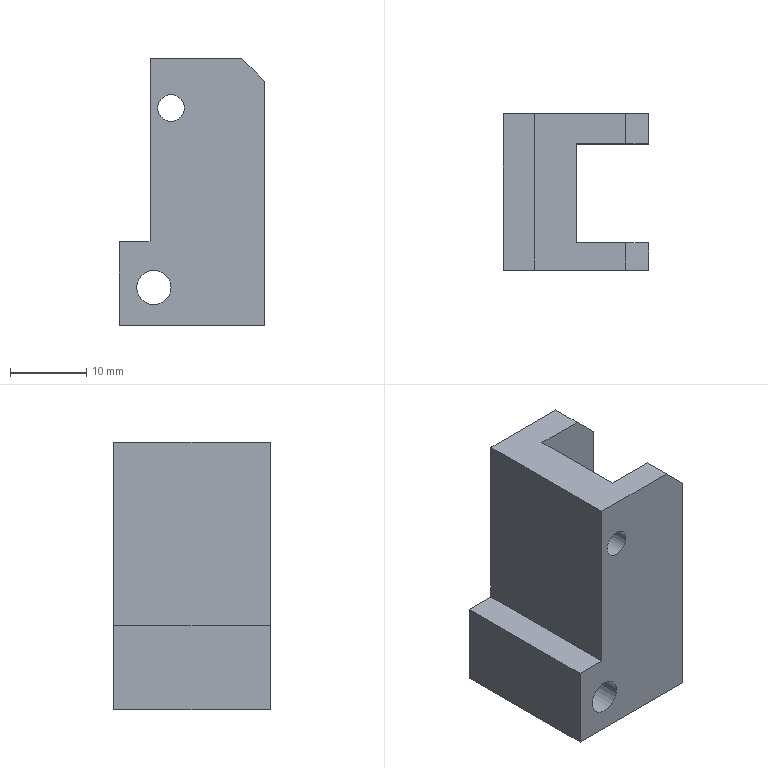Part | NX | 1 solid | 18 faces | box 19 x 20.5 x 35 mm | volume 6785 mm3 | plane 14 | cylinder 4 | commonest cylinder face diameters 3.5 x2 4.5 x2
STEP:
#1=CARTESIAN_POINT('',(9.5,16.55,0.));
#2=VERTEX_POINT('',#1);
#3=CARTESIAN_POINT('',(19.,16.55,0.));
#4=VERTEX_POINT('',#3);
#5=CARTESIAN_POINT('',(9.5,16.55,0.));
#6=DIRECTION('',(1.,0.,0.));
#7=VECTOR('',#6,1000.);
#8=LINE('',#5,#7);
#9=EDGE_CURVE('',#2,#4,#8,.T.);
#10=ORIENTED_EDGE('',*,*,#9,.F.);
#11=CARTESIAN_POINT('',(9.5,3.55,0.));
#12=VERTEX_POINT('',#11);
#13=CARTESIAN_POINT('',(9.5,3.55,0.));
#14=DIRECTION('',(0.,1.,0.));
#15=VECTOR('',#14,1000.);
#16=LINE('',#13,#15);
#17=EDGE_CURVE('',#12,#2,#16,.T.);
#18=ORIENTED_EDGE('',*,*,#17,.F.);
#19=CARTESIAN_POINT('',(19.,3.55,0.));
#20=VERTEX_POINT('',#19);
#21=CARTESIAN_POINT('',(9.5,3.55,0.));
#22=DIRECTION('',(1.,0.,0.));
#23=VECTOR('',#22,1000.);
#24=LINE('',#21,#23);
#25=EDGE_CURVE('',#12,#20,#24,.T.);
#26=ORIENTED_EDGE('',*,*,#25,.T.);
#27=CARTESIAN_POINT('',(19.,0.,0.));
#28=VERTEX_POINT('',#27);
#29=CARTESIAN_POINT('',(19.,3.55,0.));
#30=DIRECTION('',(0.,-1.,0.));
#31=VECTOR('',#30,1000.);
#32=LINE('',#29,#31);
#33=EDGE_CURVE('',#20,#28,#32,.T.);
#34=ORIENTED_EDGE('',*,*,#33,.T.);
#35=CARTESIAN_POINT('',(0.,0.,0.));
#36=VERTEX_POINT('',#35);
#37=CARTESIAN_POINT('',(19.,0.,0.));
#38=DIRECTION('',(-1.,0.,0.));
#39=VECTOR('',#38,1000.);
#40=LINE('',#37,#39);
#41=EDGE_CURVE('',#28,#36,#40,.T.);
#42=ORIENTED_EDGE('',*,*,#41,.T.);
#43=CARTESIAN_POINT('',(0.,20.5,0.));
#44=VERTEX_POINT('',#43);
#45=CARTESIAN_POINT('',(0.,0.,0.));
#46=DIRECTION('',(0.,1.,0.));
#47=VECTOR('',#46,1000.);
#48=LINE('',#45,#47);
#49=EDGE_CURVE('',#36,#44,#48,.T.);
#50=ORIENTED_EDGE('',*,*,#49,.T.);
#51=CARTESIAN_POINT('',(19.,20.5,0.));
#52=VERTEX_POINT('',#51);
#53=CARTESIAN_POINT('',(0.,20.5,0.));
#54=DIRECTION('',(1.,0.,0.));
#55=VECTOR('',#54,1000.);
#56=LINE('',#53,#55);
#57=EDGE_CURVE('',#44,#52,#56,.T.);
#58=ORIENTED_EDGE('',*,*,#57,.T.);
#59=CARTESIAN_POINT('',(19.,20.5,0.));
#60=DIRECTION('',(0.,-1.,0.));
#61=VECTOR('',#60,1000.);
#62=LINE('',#59,#61);
#63=EDGE_CURVE('',#52,#4,#62,.T.);
#64=ORIENTED_EDGE('',*,*,#63,.T.);
#65=EDGE_LOOP('',(#10,#18,#26,#34,#42,#50,#58,#64));
#66=FACE_BOUND('',#65,.T.);
#67=CARTESIAN_POINT('',(0.,0.,0.));
#68=DIRECTION('',(0.,0.,1.));
#69=DIRECTION('',(1.,0.,0.));
#70=AXIS2_PLACEMENT_3D('',#67,#68,#69);
#71=PLANE('',#70);
#72=ADVANCED_FACE('',(#66),#71,.F.);
#73=ORIENTED_EDGE('',*,*,#9,.T.);
#74=CARTESIAN_POINT('',(19.,16.55,32.));
#75=VERTEX_POINT('',#74);
#76=CARTESIAN_POINT('',(19.,16.55,32.));
#77=DIRECTION('',(0.,0.,-1.));
#78=VECTOR('',#77,1000.);
#79=LINE('',#76,#78);
#80=EDGE_CURVE('',#75,#4,#79,.T.);
#81=ORIENTED_EDGE('',*,*,#80,.F.);
#82=CARTESIAN_POINT('',(16.,16.55,35.));
#83=VERTEX_POINT('',#82);
#84=CARTESIAN_POINT('',(16.,16.55,35.));
#85=DIRECTION('',(0.7071,0.,-0.7071));
#86=VECTOR('',#85,1000.);
#87=LINE('',#84,#86);
#88=EDGE_CURVE('',#83,#75,#87,.T.);
#89=ORIENTED_EDGE('',*,*,#88,.F.);
#90=CARTESIAN_POINT('',(9.5,16.55,35.));
#91=VERTEX_POINT('',#90);
#92=CARTESIAN_POINT('',(9.5,16.55,35.));
#93=DIRECTION('',(1.,0.,0.));
#94=VECTOR('',#93,1000.);
#95=LINE('',#92,#94);
#96=EDGE_CURVE('',#91,#83,#95,.T.);
#97=ORIENTED_EDGE('',*,*,#96,.F.);
#98=CARTESIAN_POINT('',(9.5,16.55,0.));
#99=DIRECTION('',(0.,0.,1.));
#100=VECTOR('',#99,1000.);
#101=LINE('',#98,#100);
#102=EDGE_CURVE('',#2,#91,#101,.T.);
#103=ORIENTED_EDGE('',*,*,#102,.F.);
#104=EDGE_LOOP('',(#73,#81,#89,#97,#103));
#105=FACE_BOUND('',#104,.T.);
#106=CARTESIAN_POINT('',(19.,16.55,35.));
#107=DIRECTION('',(0.,1.,0.));
#108=DIRECTION('',(1.,0.,0.));
#109=AXIS2_PLACEMENT_3D('',#106,#107,#108);
#110=PLANE('',#109);
#111=ADVANCED_FACE('',(#105),#110,.F.);
#112=ORIENTED_EDGE('',*,*,#17,.T.);
#113=ORIENTED_EDGE('',*,*,#102,.T.);
#114=CARTESIAN_POINT('',(9.5,3.55,35.));
#115=VERTEX_POINT('',#114);
#116=CARTESIAN_POINT('',(9.5,3.55,35.));
#117=DIRECTION('',(0.,1.,0.));
#118=VECTOR('',#117,1000.);
#119=LINE('',#116,#118);
#120=EDGE_CURVE('',#115,#91,#119,.T.);
#121=ORIENTED_EDGE('',*,*,#120,.F.);
#122=CARTESIAN_POINT('',(9.5,3.55,0.));
#123=DIRECTION('',(0.,0.,1.));
#124=VECTOR('',#123,1000.);
#125=LINE('',#122,#124);
#126=EDGE_CURVE('',#12,#115,#125,.T.);
#127=ORIENTED_EDGE('',*,*,#126,.F.);
#128=EDGE_LOOP('',(#112,#113,#121,#127));
#129=FACE_BOUND('',#128,.T.);
#130=CARTESIAN_POINT('',(9.5,16.55,35.));
#131=DIRECTION('',(-1.,0.,0.));
#132=DIRECTION('',(0.,0.,1.));
#133=AXIS2_PLACEMENT_3D('',#130,#131,#132);
#134=PLANE('',#133);
#135=ADVANCED_FACE('',(#129),#134,.F.);
#136=ORIENTED_EDGE('',*,*,#25,.F.);
#137=ORIENTED_EDGE('',*,*,#126,.T.);
#138=CARTESIAN_POINT('',(16.,3.55,35.));
#139=VERTEX_POINT('',#138);
#140=CARTESIAN_POINT('',(9.5,3.55,35.));
#141=DIRECTION('',(1.,0.,0.));
#142=VECTOR('',#141,1000.);
#143=LINE('',#140,#142);
#144=EDGE_CURVE('',#115,#139,#143,.T.);
#145=ORIENTED_EDGE('',*,*,#144,.T.);
#146=CARTESIAN_POINT('',(19.,3.55,32.));
#147=VERTEX_POINT('',#146);
#148=CARTESIAN_POINT('',(19.,3.55,32.));
#149=DIRECTION('',(-0.7071,0.,0.7071));
#150=VECTOR('',#149,1000.);
#151=LINE('',#148,#150);
#152=EDGE_CURVE('',#147,#139,#151,.T.);
#153=ORIENTED_EDGE('',*,*,#152,.F.);
#154=CARTESIAN_POINT('',(19.,3.55,32.));
#155=DIRECTION('',(0.,0.,-1.));
#156=VECTOR('',#155,1000.);
#157=LINE('',#154,#156);
#158=EDGE_CURVE('',#147,#20,#157,.T.);
#159=ORIENTED_EDGE('',*,*,#158,.T.);
#160=EDGE_LOOP('',(#136,#137,#145,#153,#159));
#161=FACE_BOUND('',#160,.T.);
#162=CARTESIAN_POINT('',(9.5,3.55,35.));
#163=DIRECTION('',(0.,-1.,0.));
#164=DIRECTION('',(0.,0.,-1.));
#165=AXIS2_PLACEMENT_3D('',#162,#163,#164);
#166=PLANE('',#165);
#167=ADVANCED_FACE('',(#161),#166,.F.);
#168=ORIENTED_EDGE('',*,*,#158,.F.);
#169=CARTESIAN_POINT('',(19.,0.,32.));
#170=VERTEX_POINT('',#169);
#171=CARTESIAN_POINT('',(19.,3.55,32.));
#172=DIRECTION('',(0.,-1.,0.));
#173=VECTOR('',#172,1000.);
#174=LINE('',#171,#173);
#175=EDGE_CURVE('',#147,#170,#174,.T.);
#176=ORIENTED_EDGE('',*,*,#175,.T.);
#177=CARTESIAN_POINT('',(19.,0.,32.));
#178=DIRECTION('',(0.,0.,-1.));
#179=VECTOR('',#178,1000.);
#180=LINE('',#177,#179);
#181=EDGE_CURVE('',#170,#28,#180,.T.);
#182=ORIENTED_EDGE('',*,*,#181,.T.);
#183=ORIENTED_EDGE('',*,*,#33,.F.);
#184=EDGE_LOOP('',(#168,#176,#182,#183));
#185=FACE_BOUND('',#184,.T.);
#186=CARTESIAN_POINT('',(19.,0.,0.));
#187=DIRECTION('',(1.,0.,0.));
#188=DIRECTION('',(0.,1.,0.));
#189=AXIS2_PLACEMENT_3D('',#186,#187,#188);
#190=PLANE('',#189);
#191=ADVANCED_FACE('',(#185),#190,.T.);
#192=CARTESIAN_POINT('',(4.,0.,11.));
#193=VERTEX_POINT('',#192);
#194=CARTESIAN_POINT('',(4.,0.,35.));
#195=VERTEX_POINT('',#194);
#196=CARTESIAN_POINT('',(4.,0.,11.));
#197=DIRECTION('',(0.,0.,1.));
#198=VECTOR('',#197,1000.);
#199=LINE('',#196,#198);
#200=EDGE_CURVE('',#193,#195,#199,.T.);
#201=ORIENTED_EDGE('',*,*,#200,.F.);
#202=CARTESIAN_POINT('',(0.,0.,11.));
#203=VERTEX_POINT('',#202);
#204=CARTESIAN_POINT('',(4.,0.,11.));
#205=DIRECTION('',(-1.,0.,0.));
#206=VECTOR('',#205,1000.);
#207=LINE('',#204,#206);
#208=EDGE_CURVE('',#193,#203,#207,.T.);
#209=ORIENTED_EDGE('',*,*,#208,.T.);
#210=CARTESIAN_POINT('',(0.,0.,11.));
#211=DIRECTION('',(0.,0.,-1.));
#212=VECTOR('',#211,1000.);
#213=LINE('',#210,#212);
#214=EDGE_CURVE('',#203,#36,#213,.T.);
#215=ORIENTED_EDGE('',*,*,#214,.T.);
#216=ORIENTED_EDGE('',*,*,#41,.F.);
#217=ORIENTED_EDGE('',*,*,#181,.F.);
#218=CARTESIAN_POINT('',(16.,0.,35.));
#219=VERTEX_POINT('',#218);
#220=CARTESIAN_POINT('',(16.,0.,35.));
#221=DIRECTION('',(0.7071,0.,-0.7071));
#222=VECTOR('',#221,1000.);
#223=LINE('',#220,#222);
#224=EDGE_CURVE('',#219,#170,#223,.T.);
#225=ORIENTED_EDGE('',*,*,#224,.F.);
#226=CARTESIAN_POINT('',(16.,0.,35.));
#227=DIRECTION('',(-1.,0.,0.));
#228=VECTOR('',#227,1000.);
#229=LINE('',#226,#228);
#230=EDGE_CURVE('',#219,#195,#229,.T.);
#231=ORIENTED_EDGE('',*,*,#230,.T.);
#232=EDGE_LOOP('',(#201,#209,#215,#216,#217,#225,#231));
#233=FACE_BOUND('',#232,.T.);
#234=CARTESIAN_POINT('',(8.5,0.,28.5));
#235=VERTEX_POINT('',#234);
#236=CARTESIAN_POINT('',(5.,0.,28.5));
#237=VERTEX_POINT('',#236);
#238=CARTESIAN_POINT('',(6.75,0.,28.5));
#239=DIRECTION('',(0.,-1.,0.));
#240=DIRECTION('',(-1.,0.,0.));
#241=AXIS2_PLACEMENT_3D('',#238,#239,#240);
#242=CIRCLE('',#241,1.75);
#243=EDGE_CURVE('',#235,#237,#242,.T.);
#244=ORIENTED_EDGE('',*,*,#243,.F.);
#245=CARTESIAN_POINT('',(6.75,0.,28.5));
#246=DIRECTION('',(0.,-1.,0.));
#247=DIRECTION('',(-1.,0.,0.));
#248=AXIS2_PLACEMENT_3D('',#245,#246,#247);
#249=CIRCLE('',#248,1.75);
#250=EDGE_CURVE('',#237,#235,#249,.T.);
#251=ORIENTED_EDGE('',*,*,#250,.F.);
#252=EDGE_LOOP('',(#244,#251));
#253=FACE_BOUND('',#252,.T.);
#254=CARTESIAN_POINT('',(2.25,0.,5.));
#255=VERTEX_POINT('',#254);
#256=CARTESIAN_POINT('',(6.75,0.,5.));
#257=VERTEX_POINT('',#256);
#258=CARTESIAN_POINT('',(4.5,0.,5.));
#259=DIRECTION('',(0.,-1.,0.));
#260=DIRECTION('',(-1.,0.,0.));
#261=AXIS2_PLACEMENT_3D('',#258,#259,#260);
#262=CIRCLE('',#261,2.25);
#263=EDGE_CURVE('',#255,#257,#262,.T.);
#264=ORIENTED_EDGE('',*,*,#263,.F.);
#265=CARTESIAN_POINT('',(4.5,0.,5.));
#266=DIRECTION('',(0.,-1.,0.));
#267=DIRECTION('',(-1.,0.,0.));
#268=AXIS2_PLACEMENT_3D('',#265,#266,#267);
#269=CIRCLE('',#268,2.25);
#270=EDGE_CURVE('',#257,#255,#269,.T.);
#271=ORIENTED_EDGE('',*,*,#270,.F.);
#272=EDGE_LOOP('',(#264,#271));
#273=FACE_BOUND('',#272,.T.);
#274=CARTESIAN_POINT('',(0.,0.,0.));
#275=DIRECTION('',(0.,-1.,0.));
#276=DIRECTION('',(0.,0.,-1.));
#277=AXIS2_PLACEMENT_3D('',#274,#275,#276);
#278=PLANE('',#277);
#279=ADVANCED_FACE('',(#233,#253,#273),#278,.T.);
#280=CARTESIAN_POINT('',(4.,20.5,35.));
#281=VERTEX_POINT('',#280);
#282=CARTESIAN_POINT('',(4.,20.5,35.));
#283=DIRECTION('',(0.,-1.,0.));
#284=VECTOR('',#283,1000.);
#285=LINE('',#282,#284);
#286=EDGE_CURVE('',#281,#195,#285,.T.);
#287=ORIENTED_EDGE('',*,*,#286,.F.);
#288=CARTESIAN_POINT('',(4.,20.5,11.));
#289=VERTEX_POINT('',#288);
#290=CARTESIAN_POINT('',(4.,20.5,11.));
#291=DIRECTION('',(0.,0.,1.));
#292=VECTOR('',#291,1000.);
#293=LINE('',#290,#292);
#294=EDGE_CURVE('',#289,#281,#293,.T.);
#295=ORIENTED_EDGE('',*,*,#294,.F.);
#296=CARTESIAN_POINT('',(4.,0.,11.));
#297=DIRECTION('',(0.,1.,0.));
#298=VECTOR('',#297,1000.);
#299=LINE('',#296,#298);
#300=EDGE_CURVE('',#193,#289,#299,.T.);
#301=ORIENTED_EDGE('',*,*,#300,.F.);
#302=ORIENTED_EDGE('',*,*,#200,.T.);
#303=EDGE_LOOP('',(#287,#295,#301,#302));
#304=FACE_BOUND('',#303,.T.);
#305=CARTESIAN_POINT('',(4.,20.5,35.));
#306=DIRECTION('',(1.,0.,0.));
#307=DIRECTION('',(0.,1.,0.));
#308=AXIS2_PLACEMENT_3D('',#305,#306,#307);
#309=PLANE('',#308);
#310=ADVANCED_FACE('',(#304),#309,.F.);
#311=ORIENTED_EDGE('',*,*,#286,.T.);
#312=ORIENTED_EDGE('',*,*,#230,.F.);
#313=CARTESIAN_POINT('',(16.,3.55,35.));
#314=DIRECTION('',(0.,-1.,0.));
#315=VECTOR('',#314,1000.);
#316=LINE('',#313,#315);
#317=EDGE_CURVE('',#139,#219,#316,.T.);
#318=ORIENTED_EDGE('',*,*,#317,.F.);
#319=ORIENTED_EDGE('',*,*,#144,.F.);
#320=ORIENTED_EDGE('',*,*,#120,.T.);
#321=ORIENTED_EDGE('',*,*,#96,.T.);
#322=CARTESIAN_POINT('',(16.,20.5,35.));
#323=VERTEX_POINT('',#322);
#324=CARTESIAN_POINT('',(16.,20.5,35.));
#325=DIRECTION('',(0.,-1.,0.));
#326=VECTOR('',#325,1000.);
#327=LINE('',#324,#326);
#328=EDGE_CURVE('',#323,#83,#327,.T.);
#329=ORIENTED_EDGE('',*,*,#328,.F.);
#330=CARTESIAN_POINT('',(4.,20.5,35.));
#331=DIRECTION('',(1.,0.,0.));
#332=VECTOR('',#331,1000.);
#333=LINE('',#330,#332);
#334=EDGE_CURVE('',#281,#323,#333,.T.);
#335=ORIENTED_EDGE('',*,*,#334,.F.);
#336=EDGE_LOOP('',(#311,#312,#318,#319,#320,#321,#329,#335));
#337=FACE_BOUND('',#336,.T.);
#338=CARTESIAN_POINT('',(0.,0.,35.));
#339=DIRECTION('',(0.,0.,1.));
#340=DIRECTION('',(1.,0.,0.));
#341=AXIS2_PLACEMENT_3D('',#338,#339,#340);
#342=PLANE('',#341);
#343=ADVANCED_FACE('',(#337),#342,.T.);
#344=ORIENTED_EDGE('',*,*,#294,.T.);
#345=ORIENTED_EDGE('',*,*,#334,.T.);
#346=CARTESIAN_POINT('',(19.,20.5,32.));
#347=VERTEX_POINT('',#346);
#348=CARTESIAN_POINT('',(19.,20.5,32.));
#349=DIRECTION('',(-0.7071,0.,0.7071));
#350=VECTOR('',#349,1000.);
#351=LINE('',#348,#350);
#352=EDGE_CURVE('',#347,#323,#351,.T.);
#353=ORIENTED_EDGE('',*,*,#352,.F.);
#354=CARTESIAN_POINT('',(19.,20.5,32.));
#355=DIRECTION('',(0.,0.,-1.));
#356=VECTOR('',#355,1000.);
#357=LINE('',#354,#356);
#358=EDGE_CURVE('',#347,#52,#357,.T.);
#359=ORIENTED_EDGE('',*,*,#358,.T.);
#360=ORIENTED_EDGE('',*,*,#57,.F.);
#361=CARTESIAN_POINT('',(0.,20.5,11.));
#362=VERTEX_POINT('',#361);
#363=CARTESIAN_POINT('',(0.,20.5,11.));
#364=DIRECTION('',(0.,0.,-1.));
#365=VECTOR('',#364,1000.);
#366=LINE('',#363,#365);
#367=EDGE_CURVE('',#362,#44,#366,.T.);
#368=ORIENTED_EDGE('',*,*,#367,.F.);
#369=CARTESIAN_POINT('',(4.,20.5,11.));
#370=DIRECTION('',(-1.,0.,0.));
#371=VECTOR('',#370,1000.);
#372=LINE('',#369,#371);
#373=EDGE_CURVE('',#289,#362,#372,.T.);
#374=ORIENTED_EDGE('',*,*,#373,.F.);
#375=EDGE_LOOP('',(#344,#345,#353,#359,#360,#368,#374));
#376=FACE_BOUND('',#375,.T.);
#377=CARTESIAN_POINT('',(5.,20.5,28.5));
#378=VERTEX_POINT('',#377);
#379=CARTESIAN_POINT('',(8.5,20.5,28.5));
#380=VERTEX_POINT('',#379);
#381=CARTESIAN_POINT('',(6.75,20.5,28.5));
#382=DIRECTION('',(0.,1.,0.));
#383=DIRECTION('',(1.,0.,0.));
#384=AXIS2_PLACEMENT_3D('',#381,#382,#383);
#385=CIRCLE('',#384,1.75);
#386=EDGE_CURVE('',#378,#380,#385,.T.);
#387=ORIENTED_EDGE('',*,*,#386,.F.);
#388=CARTESIAN_POINT('',(6.75,20.5,28.5));
#389=DIRECTION('',(0.,1.,0.));
#390=DIRECTION('',(1.,0.,0.));
#391=AXIS2_PLACEMENT_3D('',#388,#389,#390);
#392=CIRCLE('',#391,1.75);
#393=EDGE_CURVE('',#380,#378,#392,.T.);
#394=ORIENTED_EDGE('',*,*,#393,.F.);
#395=EDGE_LOOP('',(#387,#394));
#396=FACE_BOUND('',#395,.T.);
#397=CARTESIAN_POINT('',(6.75,20.5,5.));
#398=VERTEX_POINT('',#397);
#399=CARTESIAN_POINT('',(2.25,20.5,5.));
#400=VERTEX_POINT('',#399);
#401=CARTESIAN_POINT('',(4.5,20.5,5.));
#402=DIRECTION('',(0.,1.,0.));
#403=DIRECTION('',(1.,0.,0.));
#404=AXIS2_PLACEMENT_3D('',#401,#402,#403);
#405=CIRCLE('',#404,2.25);
#406=EDGE_CURVE('',#398,#400,#405,.T.);
#407=ORIENTED_EDGE('',*,*,#406,.F.);
#408=CARTESIAN_POINT('',(4.5,20.5,5.));
#409=DIRECTION('',(0.,1.,0.));
#410=DIRECTION('',(1.,0.,0.));
#411=AXIS2_PLACEMENT_3D('',#408,#409,#410);
#412=CIRCLE('',#411,2.25);
#413=EDGE_CURVE('',#400,#398,#412,.T.);
#414=ORIENTED_EDGE('',*,*,#413,.F.);
#415=EDGE_LOOP('',(#407,#414));
#416=FACE_BOUND('',#415,.T.);
#417=CARTESIAN_POINT('',(19.,20.5,0.));
#418=DIRECTION('',(0.,1.,0.));
#419=DIRECTION('',(1.,0.,0.));
#420=AXIS2_PLACEMENT_3D('',#417,#418,#419);
#421=PLANE('',#420);
#422=ADVANCED_FACE('',(#376,#396,#416),#421,.T.);
#423=ORIENTED_EDGE('',*,*,#208,.F.);
#424=ORIENTED_EDGE('',*,*,#300,.T.);
#425=ORIENTED_EDGE('',*,*,#373,.T.);
#426=CARTESIAN_POINT('',(0.,0.,11.));
#427=DIRECTION('',(0.,1.,0.));
#428=VECTOR('',#427,1000.);
#429=LINE('',#426,#428);
#430=EDGE_CURVE('',#203,#362,#429,.T.);
#431=ORIENTED_EDGE('',*,*,#430,.F.);
#432=EDGE_LOOP('',(#423,#424,#425,#431));
#433=FACE_BOUND('',#432,.T.);
#434=CARTESIAN_POINT('',(4.,20.5,11.));
#435=DIRECTION('',(0.,0.,-1.));
#436=DIRECTION('',(0.,-1.,0.));
#437=AXIS2_PLACEMENT_3D('',#434,#435,#436);
#438=PLANE('',#437);
#439=ADVANCED_FACE('',(#433),#438,.F.);
#440=ORIENTED_EDGE('',*,*,#430,.T.);
#441=ORIENTED_EDGE('',*,*,#367,.T.);
#442=ORIENTED_EDGE('',*,*,#49,.F.);
#443=ORIENTED_EDGE('',*,*,#214,.F.);
#444=EDGE_LOOP('',(#440,#441,#442,#443));
#445=FACE_BOUND('',#444,.T.);
#446=CARTESIAN_POINT('',(0.,20.5,0.));
#447=DIRECTION('',(-1.,0.,0.));
#448=DIRECTION('',(0.,0.,1.));
#449=AXIS2_PLACEMENT_3D('',#446,#447,#448);
#450=PLANE('',#449);
#451=ADVANCED_FACE('',(#445),#450,.T.);
#452=ORIENTED_EDGE('',*,*,#80,.T.);
#453=ORIENTED_EDGE('',*,*,#63,.F.);
#454=ORIENTED_EDGE('',*,*,#358,.F.);
#455=CARTESIAN_POINT('',(19.,20.5,32.));
#456=DIRECTION('',(0.,-1.,0.));
#457=VECTOR('',#456,1000.);
#458=LINE('',#455,#457);
#459=EDGE_CURVE('',#347,#75,#458,.T.);
#460=ORIENTED_EDGE('',*,*,#459,.T.);
#461=EDGE_LOOP('',(#452,#453,#454,#460));
#462=FACE_BOUND('',#461,.T.);
#463=CARTESIAN_POINT('',(19.,0.,0.));
#464=DIRECTION('',(1.,0.,0.));
#465=DIRECTION('',(0.,1.,0.));
#466=AXIS2_PLACEMENT_3D('',#463,#464,#465);
#467=PLANE('',#466);
#468=ADVANCED_FACE('',(#462),#467,.T.);
#469=ORIENTED_EDGE('',*,*,#328,.T.);
#470=ORIENTED_EDGE('',*,*,#88,.T.);
#471=ORIENTED_EDGE('',*,*,#459,.F.);
#472=ORIENTED_EDGE('',*,*,#352,.T.);
#473=EDGE_LOOP('',(#469,#470,#471,#472));
#474=FACE_BOUND('',#473,.T.);
#475=CARTESIAN_POINT('',(16.,16.55,35.));
#476=DIRECTION('',(-0.7071,0.,-0.7071));
#477=DIRECTION('',(-0.7071,0.,0.7071));
#478=AXIS2_PLACEMENT_3D('',#475,#476,#477);
#479=PLANE('',#478);
#480=ADVANCED_FACE('',(#474),#479,.F.);
#481=ORIENTED_EDGE('',*,*,#386,.T.);
#482=CARTESIAN_POINT('',(8.5,20.5,28.5));
#483=DIRECTION('',(0.,-1.,0.));
#484=VECTOR('',#483,1000.);
#485=LINE('',#482,#484);
#486=EDGE_CURVE('',#380,#235,#485,.T.);
#487=ORIENTED_EDGE('',*,*,#486,.T.);
#488=ORIENTED_EDGE('',*,*,#243,.T.);
#489=CARTESIAN_POINT('',(5.,20.5,28.5));
#490=DIRECTION('',(0.,-1.,0.));
#491=VECTOR('',#490,1000.);
#492=LINE('',#489,#491);
#493=EDGE_CURVE('',#378,#237,#492,.T.);
#494=ORIENTED_EDGE('',*,*,#493,.F.);
#495=EDGE_LOOP('',(#481,#487,#488,#494));
#496=FACE_BOUND('',#495,.T.);
#497=CARTESIAN_POINT('',(6.75,20.5,28.5));
#498=DIRECTION('',(0.,-1.,0.));
#499=DIRECTION('',(1.,0.,0.));
#500=AXIS2_PLACEMENT_3D('',#497,#498,#499);
#501=CYLINDRICAL_SURFACE('',#500,1.75);
#502=ADVANCED_FACE('',(#496),#501,.F.);
#503=ORIENTED_EDGE('',*,*,#317,.T.);
#504=ORIENTED_EDGE('',*,*,#224,.T.);
#505=ORIENTED_EDGE('',*,*,#175,.F.);
#506=ORIENTED_EDGE('',*,*,#152,.T.);
#507=EDGE_LOOP('',(#503,#504,#505,#506));
#508=FACE_BOUND('',#507,.T.);
#509=CARTESIAN_POINT('',(16.,0.,35.));
#510=DIRECTION('',(-0.7071,0.,-0.7071));
#511=DIRECTION('',(-0.7071,0.,0.7071));
#512=AXIS2_PLACEMENT_3D('',#509,#510,#511);
#513=PLANE('',#512);
#514=ADVANCED_FACE('',(#508),#513,.F.);
#515=ORIENTED_EDGE('',*,*,#263,.T.);
#516=CARTESIAN_POINT('',(6.75,20.5,5.));
#517=DIRECTION('',(0.,-1.,0.));
#518=VECTOR('',#517,1000.);
#519=LINE('',#516,#518);
#520=EDGE_CURVE('',#398,#257,#519,.T.);
#521=ORIENTED_EDGE('',*,*,#520,.F.);
#522=ORIENTED_EDGE('',*,*,#406,.T.);
#523=CARTESIAN_POINT('',(2.25,20.5,5.));
#524=DIRECTION('',(0.,-1.,0.));
#525=VECTOR('',#524,1000.);
#526=LINE('',#523,#525);
#527=EDGE_CURVE('',#400,#255,#526,.T.);
#528=ORIENTED_EDGE('',*,*,#527,.T.);
#529=EDGE_LOOP('',(#515,#521,#522,#528));
#530=FACE_BOUND('',#529,.T.);
#531=CARTESIAN_POINT('',(4.5,20.5,5.));
#532=DIRECTION('',(0.,-1.,0.));
#533=DIRECTION('',(1.,0.,0.));
#534=AXIS2_PLACEMENT_3D('',#531,#532,#533);
#535=CYLINDRICAL_SURFACE('',#534,2.25);
#536=ADVANCED_FACE('',(#530),#535,.F.);
#537=ORIENTED_EDGE('',*,*,#486,.F.);
#538=ORIENTED_EDGE('',*,*,#393,.T.);
#539=ORIENTED_EDGE('',*,*,#493,.T.);
#540=ORIENTED_EDGE('',*,*,#250,.T.);
#541=EDGE_LOOP('',(#537,#538,#539,#540));
#542=FACE_BOUND('',#541,.T.);
#543=CARTESIAN_POINT('',(6.75,20.5,28.5));
#544=DIRECTION('',(0.,-1.,0.));
#545=DIRECTION('',(1.,0.,0.));
#546=AXIS2_PLACEMENT_3D('',#543,#544,#545);
#547=CYLINDRICAL_SURFACE('',#546,1.75);
#548=ADVANCED_FACE('',(#542),#547,.F.);
#549=ORIENTED_EDGE('',*,*,#520,.T.);
#550=ORIENTED_EDGE('',*,*,#270,.T.);
#551=ORIENTED_EDGE('',*,*,#527,.F.);
#552=ORIENTED_EDGE('',*,*,#413,.T.);
#553=EDGE_LOOP('',(#549,#550,#551,#552));
#554=FACE_BOUND('',#553,.T.);
#555=CARTESIAN_POINT('',(4.5,20.5,5.));
#556=DIRECTION('',(0.,-1.,0.));
#557=DIRECTION('',(1.,0.,0.));
#558=AXIS2_PLACEMENT_3D('',#555,#556,#557);
#559=CYLINDRICAL_SURFACE('',#558,2.25);
#560=ADVANCED_FACE('',(#554),#559,.F.);
#561=CLOSED_SHELL('',(#72,#111,#135,#167,#191,#279,#310,#343,#422,#439,#451,#468,#480,#502,#514,#536,#548,#560));
#562=MANIFOLD_SOLID_BREP('',#561);
#563=(LENGTH_UNIT()NAMED_UNIT(*)SI_UNIT(.MILLI.,.METRE.));
#564=UNCERTAINTY_MEASURE_WITH_UNIT(LENGTH_MEASURE(0.00001),#563,'','');
#565=(NAMED_UNIT(*)PLANE_ANGLE_UNIT()SI_UNIT($,.RADIAN.));
#566=(NAMED_UNIT(*)SI_UNIT($,.STERADIAN.)SOLID_ANGLE_UNIT());
#567=(GEOMETRIC_REPRESENTATION_CONTEXT(3)GLOBAL_UNCERTAINTY_ASSIGNED_CONTEXT((#564))GLOBAL_UNIT_ASSIGNED_CONTEXT((#563,#565,#566))REPRESENTATION_CONTEXT('',''));
#568=ADVANCED_BREP_SHAPE_REPRESENTATION('',(#562),#567);